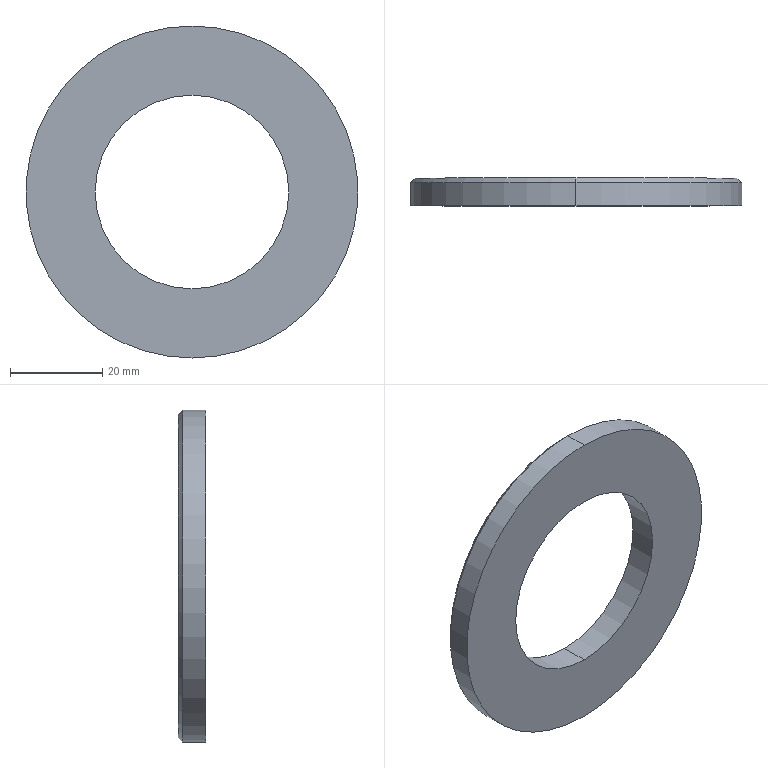Part | SolidWorks | features Revolution 1 | 1 solid | 8 faces | box 72 x 6 x 72 mm | volume 16004 mm3 | cylinder 4 | cone 2 | plane 2 | commonest cylinder face diameters 42 x2 72 x2
STEP:
#1=CARTESIAN_POINT('',(0.,13.645,-36.));
#2=VERTEX_POINT('',#1);
#3=CARTESIAN_POINT('',(0.,13.645,36.));
#4=VERTEX_POINT('',#3);
#5=CARTESIAN_POINT('',(0.,13.645,0.));
#6=DIRECTION('',(0.,-1.,0.));
#7=DIRECTION('',(0.,0.,-1.));
#8=AXIS2_PLACEMENT_3D('',#5,#6,#7);
#9=CIRCLE('',#8,36.);
#10=EDGE_CURVE('',#2,#4,#9,.T.);
#11=ORIENTED_EDGE('',*,*,#10,.T.);
#12=CARTESIAN_POINT('',(0.,8.645,36.));
#13=VERTEX_POINT('',#12);
#14=CARTESIAN_POINT('',(0.,0.,36.));
#15=DIRECTION('',(0.,-1.,0.));
#16=VECTOR('',#15,1000.);
#17=LINE('',#14,#16);
#18=EDGE_CURVE('',#4,#13,#17,.T.);
#19=ORIENTED_EDGE('',*,*,#18,.T.);
#20=CARTESIAN_POINT('',(0.,8.645,-36.));
#21=VERTEX_POINT('',#20);
#22=CARTESIAN_POINT('',(0.,8.645,0.));
#23=DIRECTION('',(0.,-1.,0.));
#24=DIRECTION('',(0.,0.,-1.));
#25=AXIS2_PLACEMENT_3D('',#22,#23,#24);
#26=CIRCLE('',#25,36.);
#27=EDGE_CURVE('',#21,#13,#26,.T.);
#28=ORIENTED_EDGE('',*,*,#27,.F.);
#29=CARTESIAN_POINT('',(0.,0.,-36.));
#30=DIRECTION('',(0.,-1.,0.));
#31=VECTOR('',#30,1000.);
#32=LINE('',#29,#31);
#33=EDGE_CURVE('',#2,#21,#32,.T.);
#34=ORIENTED_EDGE('',*,*,#33,.F.);
#35=EDGE_LOOP('',(#11,#19,#28,#34));
#36=FACE_OUTER_BOUND('',#35,.T.);
#37=CARTESIAN_POINT('',(0.,0.,0.));
#38=DIRECTION('',(0.,-1.,0.));
#39=DIRECTION('',(0.,0.,-1.));
#40=AXIS2_PLACEMENT_3D('',#37,#38,#39);
#41=CYLINDRICAL_SURFACE('',#40,36.);
#42=ADVANCED_FACE('',(#36),#41,.T.);
#43=CARTESIAN_POINT('',(0.,14.645,-35.));
#44=VERTEX_POINT('',#43);
#45=CARTESIAN_POINT('',(0.,14.645,35.));
#46=VERTEX_POINT('',#45);
#47=CARTESIAN_POINT('',(0.,14.645,0.));
#48=DIRECTION('',(0.,-1.,0.));
#49=DIRECTION('',(0.,0.,-1.));
#50=AXIS2_PLACEMENT_3D('',#47,#48,#49);
#51=CIRCLE('',#50,35.);
#52=EDGE_CURVE('',#44,#46,#51,.T.);
#53=ORIENTED_EDGE('',*,*,#52,.T.);
#54=CARTESIAN_POINT('',(0.,14.645,35.));
#55=DIRECTION('',(0.,-0.7071,0.7071));
#56=VECTOR('',#55,1000.);
#57=LINE('',#54,#56);
#58=EDGE_CURVE('',#46,#4,#57,.T.);
#59=ORIENTED_EDGE('',*,*,#58,.T.);
#60=ORIENTED_EDGE('',*,*,#10,.F.);
#61=CARTESIAN_POINT('',(0.,14.645,-35.));
#62=DIRECTION('',(0.,-0.7071,-0.7071));
#63=VECTOR('',#62,1000.);
#64=LINE('',#61,#63);
#65=EDGE_CURVE('',#44,#2,#64,.T.);
#66=ORIENTED_EDGE('',*,*,#65,.F.);
#67=EDGE_LOOP('',(#53,#59,#60,#66));
#68=FACE_OUTER_BOUND('',#67,.T.);
#69=CARTESIAN_POINT('',(0.,14.645,0.));
#70=DIRECTION('',(0.,-1.,0.));
#71=DIRECTION('',(0.,0.,-1.));
#72=AXIS2_PLACEMENT_3D('',#69,#70,#71);
#73=CONICAL_SURFACE('',#72,35.,0.7854);
#74=ADVANCED_FACE('',(#68),#73,.T.);
#75=CARTESIAN_POINT('',(0.,14.645,21.));
#76=VERTEX_POINT('',#75);
#77=CARTESIAN_POINT('',(0.,14.645,-21.));
#78=VERTEX_POINT('',#77);
#79=CARTESIAN_POINT('',(0.,14.645,0.));
#80=DIRECTION('',(0.,-1.,0.));
#81=DIRECTION('',(0.,0.,-1.));
#82=AXIS2_PLACEMENT_3D('',#79,#80,#81);
#83=CIRCLE('',#82,21.);
#84=EDGE_CURVE('',#76,#78,#83,.T.);
#85=ORIENTED_EDGE('',*,*,#84,.F.);
#86=CARTESIAN_POINT('',(0.,8.645,21.));
#87=VERTEX_POINT('',#86);
#88=CARTESIAN_POINT('',(0.,0.,21.));
#89=DIRECTION('',(0.,-1.,0.));
#90=VECTOR('',#89,1000.);
#91=LINE('',#88,#90);
#92=EDGE_CURVE('',#76,#87,#91,.T.);
#93=ORIENTED_EDGE('',*,*,#92,.T.);
#94=CARTESIAN_POINT('',(0.,8.645,-21.));
#95=VERTEX_POINT('',#94);
#96=CARTESIAN_POINT('',(0.,8.645,0.));
#97=DIRECTION('',(0.,-1.,0.));
#98=DIRECTION('',(0.,0.,-1.));
#99=AXIS2_PLACEMENT_3D('',#96,#97,#98);
#100=CIRCLE('',#99,21.);
#101=EDGE_CURVE('',#87,#95,#100,.T.);
#102=ORIENTED_EDGE('',*,*,#101,.T.);
#103=CARTESIAN_POINT('',(0.,0.,-21.));
#104=DIRECTION('',(0.,-1.,0.));
#105=VECTOR('',#104,1000.);
#106=LINE('',#103,#105);
#107=EDGE_CURVE('',#78,#95,#106,.T.);
#108=ORIENTED_EDGE('',*,*,#107,.F.);
#109=EDGE_LOOP('',(#85,#93,#102,#108));
#110=FACE_OUTER_BOUND('',#109,.T.);
#111=CARTESIAN_POINT('',(0.,0.,0.));
#112=DIRECTION('',(0.,-1.,0.));
#113=DIRECTION('',(0.,0.,-1.));
#114=AXIS2_PLACEMENT_3D('',#111,#112,#113);
#115=CYLINDRICAL_SURFACE('',#114,21.);
#116=ADVANCED_FACE('',(#110),#115,.F.);
#117=ORIENTED_EDGE('',*,*,#92,.F.);
#118=CARTESIAN_POINT('',(0.,14.645,0.));
#119=DIRECTION('',(0.,-1.,0.));
#120=DIRECTION('',(0.,0.,-1.));
#121=AXIS2_PLACEMENT_3D('',#118,#119,#120);
#122=CIRCLE('',#121,21.);
#123=EDGE_CURVE('',#78,#76,#122,.T.);
#124=ORIENTED_EDGE('',*,*,#123,.F.);
#125=ORIENTED_EDGE('',*,*,#107,.T.);
#126=CARTESIAN_POINT('',(0.,8.645,0.));
#127=DIRECTION('',(0.,-1.,0.));
#128=DIRECTION('',(0.,0.,-1.));
#129=AXIS2_PLACEMENT_3D('',#126,#127,#128);
#130=CIRCLE('',#129,21.);
#131=EDGE_CURVE('',#95,#87,#130,.T.);
#132=ORIENTED_EDGE('',*,*,#131,.T.);
#133=EDGE_LOOP('',(#117,#124,#125,#132));
#134=FACE_OUTER_BOUND('',#133,.T.);
#135=CARTESIAN_POINT('',(0.,0.,0.));
#136=DIRECTION('',(0.,-1.,0.));
#137=DIRECTION('',(0.,0.,-1.));
#138=AXIS2_PLACEMENT_3D('',#135,#136,#137);
#139=CYLINDRICAL_SURFACE('',#138,21.);
#140=ADVANCED_FACE('',(#134),#139,.F.);
#141=ORIENTED_EDGE('',*,*,#52,.F.);
#142=CARTESIAN_POINT('',(0.,14.645,0.));
#143=DIRECTION('',(0.,-1.,0.));
#144=DIRECTION('',(0.,0.,-1.));
#145=AXIS2_PLACEMENT_3D('',#142,#143,#144);
#146=CIRCLE('',#145,35.);
#147=EDGE_CURVE('',#46,#44,#146,.T.);
#148=ORIENTED_EDGE('',*,*,#147,.F.);
#149=EDGE_LOOP('',(#141,#148));
#150=FACE_OUTER_BOUND('',#149,.T.);
#151=ORIENTED_EDGE('',*,*,#123,.T.);
#152=ORIENTED_EDGE('',*,*,#84,.T.);
#153=EDGE_LOOP('',(#151,#152));
#154=FACE_BOUND('',#153,.T.);
#155=CARTESIAN_POINT('',(-21.,14.645,0.));
#156=DIRECTION('',(0.,-1.,0.));
#157=DIRECTION('',(0.,0.,-1.));
#158=AXIS2_PLACEMENT_3D('',#155,#156,#157);
#159=PLANE('',#158);
#160=ADVANCED_FACE('',(#150,#154),#159,.F.);
#161=ORIENTED_EDGE('',*,*,#58,.F.);
#162=ORIENTED_EDGE('',*,*,#147,.T.);
#163=ORIENTED_EDGE('',*,*,#65,.T.);
#164=CARTESIAN_POINT('',(0.,13.645,0.));
#165=DIRECTION('',(0.,-1.,0.));
#166=DIRECTION('',(0.,0.,-1.));
#167=AXIS2_PLACEMENT_3D('',#164,#165,#166);
#168=CIRCLE('',#167,36.);
#169=EDGE_CURVE('',#4,#2,#168,.T.);
#170=ORIENTED_EDGE('',*,*,#169,.F.);
#171=EDGE_LOOP('',(#161,#162,#163,#170));
#172=FACE_OUTER_BOUND('',#171,.T.);
#173=CARTESIAN_POINT('',(0.,14.645,0.));
#174=DIRECTION('',(0.,-1.,0.));
#175=DIRECTION('',(0.,0.,-1.));
#176=AXIS2_PLACEMENT_3D('',#173,#174,#175);
#177=CONICAL_SURFACE('',#176,35.,0.7854);
#178=ADVANCED_FACE('',(#172),#177,.T.);
#179=ORIENTED_EDGE('',*,*,#18,.F.);
#180=ORIENTED_EDGE('',*,*,#169,.T.);
#181=ORIENTED_EDGE('',*,*,#33,.T.);
#182=CARTESIAN_POINT('',(0.,8.645,0.));
#183=DIRECTION('',(0.,-1.,0.));
#184=DIRECTION('',(0.,0.,-1.));
#185=AXIS2_PLACEMENT_3D('',#182,#183,#184);
#186=CIRCLE('',#185,36.);
#187=EDGE_CURVE('',#13,#21,#186,.T.);
#188=ORIENTED_EDGE('',*,*,#187,.F.);
#189=EDGE_LOOP('',(#179,#180,#181,#188));
#190=FACE_OUTER_BOUND('',#189,.T.);
#191=CARTESIAN_POINT('',(0.,0.,0.));
#192=DIRECTION('',(0.,-1.,0.));
#193=DIRECTION('',(0.,0.,-1.));
#194=AXIS2_PLACEMENT_3D('',#191,#192,#193);
#195=CYLINDRICAL_SURFACE('',#194,36.);
#196=ADVANCED_FACE('',(#190),#195,.T.);
#197=ORIENTED_EDGE('',*,*,#131,.F.);
#198=ORIENTED_EDGE('',*,*,#101,.F.);
#199=EDGE_LOOP('',(#197,#198));
#200=FACE_BOUND('',#199,.T.);
#201=ORIENTED_EDGE('',*,*,#27,.T.);
#202=ORIENTED_EDGE('',*,*,#187,.T.);
#203=EDGE_LOOP('',(#201,#202));
#204=FACE_OUTER_BOUND('',#203,.T.);
#205=CARTESIAN_POINT('',(-21.,8.645,0.));
#206=DIRECTION('',(0.,1.,0.));
#207=DIRECTION('',(0.,0.,1.));
#208=AXIS2_PLACEMENT_3D('',#205,#206,#207);
#209=PLANE('',#208);
#210=ADVANCED_FACE('',(#200,#204),#209,.F.);
#211=CLOSED_SHELL('',(#42,#74,#116,#140,#160,#178,#196,#210));
#212=MANIFOLD_SOLID_BREP('',#211);
#213=CARTESIAN_POINT('',(0.,0.,0.));
#214=DIRECTION('',(0.,0.,1.));
#215=DIRECTION('',(1.,0.,0.));
#216=AXIS2_PLACEMENT_3D('',#213,#214,#215);
#217=(LENGTH_UNIT()NAMED_UNIT(*)SI_UNIT(.MILLI.,.METRE.));
#218=UNCERTAINTY_MEASURE_WITH_UNIT(LENGTH_MEASURE(0.00001),#217,'','');
#219=(NAMED_UNIT(*)PLANE_ANGLE_UNIT()SI_UNIT($,.RADIAN.));
#220=(NAMED_UNIT(*)SI_UNIT($,.STERADIAN.)SOLID_ANGLE_UNIT());
#221=(GEOMETRIC_REPRESENTATION_CONTEXT(3)GLOBAL_UNCERTAINTY_ASSIGNED_CONTEXT((#218))GLOBAL_UNIT_ASSIGNED_CONTEXT((#217,#219,#220))REPRESENTATION_CONTEXT('',''));
#222=ADVANCED_BREP_SHAPE_REPRESENTATION('',(#212,#216),#221);